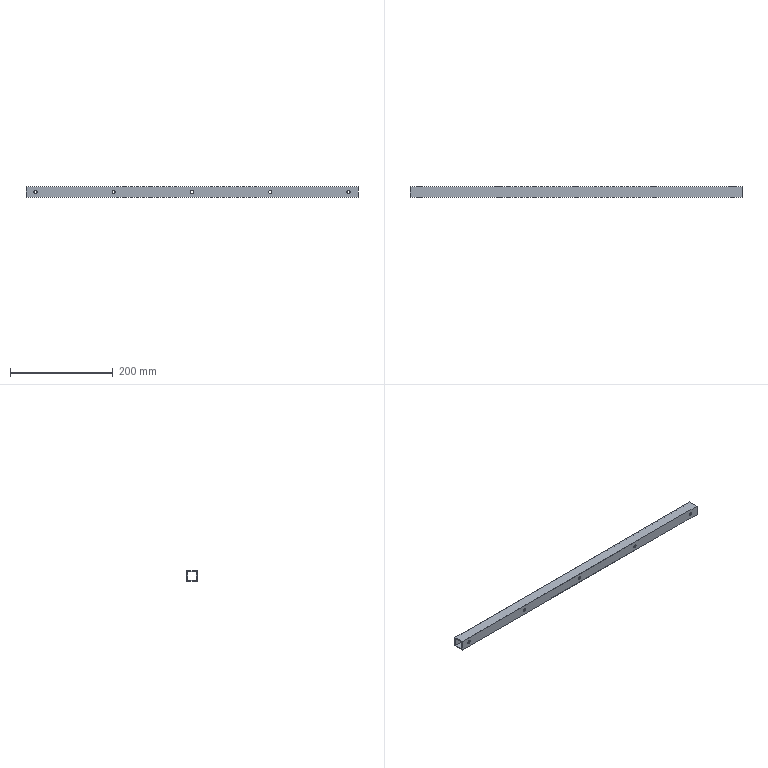Part | STEP file | 5091202 | 1 solid | 20 faces | box 645 x 20 x 20 mm | volume 70797 mm3 | plane 10 | cylinder 10 | commonest cylinder face diameters 10 x5 6 x4 5.759 x1